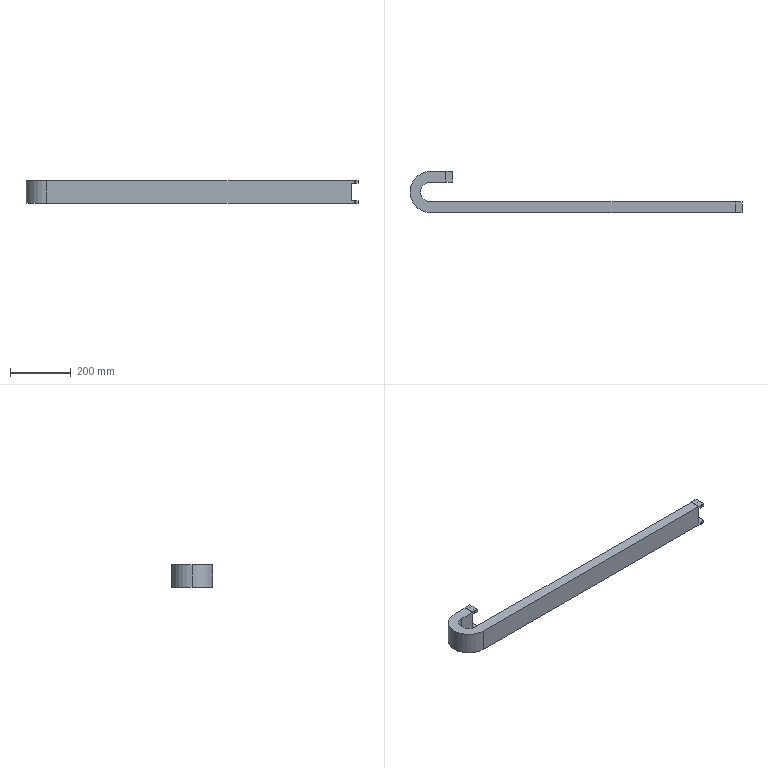Part | SolidWorks | features ICE 4, HoleWzd 2, Shell 1, Sweep 1 | 1 solid | 44 faces | box 1090 x 135 x 77 mm | volume 1433722 mm3 | plane 28 | cylinder 16 | commonest cylinder face diameters 5.5 x8 65 x2 75 x2 125 x2 135 x2
STEP:
#1=CARTESIAN_POINT('',(-938.,82.5,-36.25));
#2=VERTEX_POINT('',#1);
#3=CARTESIAN_POINT('',(-938.,82.5,-30.75));
#4=VERTEX_POINT('',#3);
#5=CARTESIAN_POINT('',(-938.,82.5,-33.5));
#6=DIRECTION('',(0.,1.,0.));
#7=DIRECTION('',(-1.,0.,0.));
#8=AXIS2_PLACEMENT_3D('',#5,#6,#7);
#9=CIRCLE('',#8,2.75);
#10=EDGE_CURVE('',#2,#4,#9,.T.);
#11=ORIENTED_EDGE('',*,*,#10,.F.);
#12=CARTESIAN_POINT('',(-938.,117.5,-36.25));
#13=VERTEX_POINT('',#12);
#14=CARTESIAN_POINT('',(-938.,117.5,-36.25));
#15=DIRECTION('',(0.,1.,0.));
#16=VECTOR('',#15,1000.);
#17=LINE('',#14,#16);
#18=EDGE_CURVE('',#2,#13,#17,.T.);
#19=ORIENTED_EDGE('',*,*,#18,.T.);
#20=CARTESIAN_POINT('',(-938.,117.5,-30.75));
#21=VERTEX_POINT('',#20);
#22=CARTESIAN_POINT('',(-938.,117.5,-33.5));
#23=DIRECTION('',(0.,1.,0.));
#24=DIRECTION('',(0.,0.,1.));
#25=AXIS2_PLACEMENT_3D('',#22,#23,#24);
#26=CIRCLE('',#25,2.75);
#27=EDGE_CURVE('',#13,#21,#26,.T.);
#28=ORIENTED_EDGE('',*,*,#27,.T.);
#29=CARTESIAN_POINT('',(-938.,117.5,-30.75));
#30=DIRECTION('',(0.,1.,0.));
#31=VECTOR('',#30,1000.);
#32=LINE('',#29,#31);
#33=EDGE_CURVE('',#4,#21,#32,.T.);
#34=ORIENTED_EDGE('',*,*,#33,.F.);
#35=EDGE_LOOP('',(#11,#19,#28,#34));
#36=FACE_OUTER_BOUND('',#35,.T.);
#37=CARTESIAN_POINT('',(-938.,117.5,-33.5));
#38=DIRECTION('',(0.,1.,0.));
#39=DIRECTION('',(0.,0.,1.));
#40=AXIS2_PLACEMENT_3D('',#37,#38,#39);
#41=CYLINDRICAL_SURFACE('',#40,2.75);
#42=ADVANCED_FACE('',(#36),#41,.F.);
#43=CARTESIAN_POINT('',(-938.,82.5,30.75));
#44=VERTEX_POINT('',#43);
#45=CARTESIAN_POINT('',(-938.,82.5,36.25));
#46=VERTEX_POINT('',#45);
#47=CARTESIAN_POINT('',(-938.,82.5,33.5));
#48=DIRECTION('',(0.,1.,0.));
#49=DIRECTION('',(-1.,0.,0.));
#50=AXIS2_PLACEMENT_3D('',#47,#48,#49);
#51=CIRCLE('',#50,2.75);
#52=EDGE_CURVE('',#44,#46,#51,.T.);
#53=ORIENTED_EDGE('',*,*,#52,.F.);
#54=CARTESIAN_POINT('',(-938.,117.5,30.75));
#55=VERTEX_POINT('',#54);
#56=CARTESIAN_POINT('',(-938.,117.5,30.75));
#57=DIRECTION('',(0.,1.,0.));
#58=VECTOR('',#57,1000.);
#59=LINE('',#56,#58);
#60=EDGE_CURVE('',#44,#55,#59,.T.);
#61=ORIENTED_EDGE('',*,*,#60,.T.);
#62=CARTESIAN_POINT('',(-938.,117.5,36.25));
#63=VERTEX_POINT('',#62);
#64=CARTESIAN_POINT('',(-938.,117.5,33.5));
#65=DIRECTION('',(0.,1.,0.));
#66=DIRECTION('',(0.,0.,1.));
#67=AXIS2_PLACEMENT_3D('',#64,#65,#66);
#68=CIRCLE('',#67,2.75);
#69=EDGE_CURVE('',#55,#63,#68,.T.);
#70=ORIENTED_EDGE('',*,*,#69,.T.);
#71=CARTESIAN_POINT('',(-938.,117.5,36.25));
#72=DIRECTION('',(0.,1.,0.));
#73=VECTOR('',#72,1000.);
#74=LINE('',#71,#73);
#75=EDGE_CURVE('',#46,#63,#74,.T.);
#76=ORIENTED_EDGE('',*,*,#75,.F.);
#77=EDGE_LOOP('',(#53,#61,#70,#76));
#78=FACE_OUTER_BOUND('',#77,.T.);
#79=CARTESIAN_POINT('',(-938.,117.5,33.5));
#80=DIRECTION('',(0.,1.,0.));
#81=DIRECTION('',(0.,0.,1.));
#82=AXIS2_PLACEMENT_3D('',#79,#80,#81);
#83=CYLINDRICAL_SURFACE('',#82,2.75);
#84=ADVANCED_FACE('',(#78),#83,.F.);
#85=CARTESIAN_POINT('',(12.,-17.5,-30.75));
#86=VERTEX_POINT('',#85);
#87=CARTESIAN_POINT('',(12.,-17.5,-36.25));
#88=VERTEX_POINT('',#87);
#89=CARTESIAN_POINT('',(12.,-17.5,-33.5));
#90=DIRECTION('',(0.,-1.,0.));
#91=DIRECTION('',(1.,0.,0.));
#92=AXIS2_PLACEMENT_3D('',#89,#90,#91);
#93=CIRCLE('',#92,2.75);
#94=EDGE_CURVE('',#86,#88,#93,.T.);
#95=ORIENTED_EDGE('',*,*,#94,.T.);
#96=CARTESIAN_POINT('',(12.,17.5,-36.25));
#97=VERTEX_POINT('',#96);
#98=CARTESIAN_POINT('',(12.,17.5,-36.25));
#99=DIRECTION('',(0.,1.,0.));
#100=VECTOR('',#99,1000.);
#101=LINE('',#98,#100);
#102=EDGE_CURVE('',#88,#97,#101,.T.);
#103=ORIENTED_EDGE('',*,*,#102,.T.);
#104=CARTESIAN_POINT('',(12.,17.5,-30.75));
#105=VERTEX_POINT('',#104);
#106=CARTESIAN_POINT('',(12.,17.5,-33.5));
#107=DIRECTION('',(0.,1.,0.));
#108=DIRECTION('',(0.,0.,1.));
#109=AXIS2_PLACEMENT_3D('',#106,#107,#108);
#110=CIRCLE('',#109,2.75);
#111=EDGE_CURVE('',#97,#105,#110,.T.);
#112=ORIENTED_EDGE('',*,*,#111,.T.);
#113=CARTESIAN_POINT('',(12.,17.5,-30.75));
#114=DIRECTION('',(0.,1.,0.));
#115=VECTOR('',#114,1000.);
#116=LINE('',#113,#115);
#117=EDGE_CURVE('',#86,#105,#116,.T.);
#118=ORIENTED_EDGE('',*,*,#117,.F.);
#119=EDGE_LOOP('',(#95,#103,#112,#118));
#120=FACE_OUTER_BOUND('',#119,.T.);
#121=CARTESIAN_POINT('',(12.,17.5,-33.5));
#122=DIRECTION('',(0.,1.,0.));
#123=DIRECTION('',(0.,0.,1.));
#124=AXIS2_PLACEMENT_3D('',#121,#122,#123);
#125=CYLINDRICAL_SURFACE('',#124,2.75);
#126=ADVANCED_FACE('',(#120),#125,.F.);
#127=CARTESIAN_POINT('',(12.,-17.5,36.25));
#128=VERTEX_POINT('',#127);
#129=CARTESIAN_POINT('',(12.,-17.5,30.75));
#130=VERTEX_POINT('',#129);
#131=CARTESIAN_POINT('',(12.,-17.5,33.5));
#132=DIRECTION('',(0.,-1.,0.));
#133=DIRECTION('',(1.,0.,0.));
#134=AXIS2_PLACEMENT_3D('',#131,#132,#133);
#135=CIRCLE('',#134,2.75);
#136=EDGE_CURVE('',#128,#130,#135,.T.);
#137=ORIENTED_EDGE('',*,*,#136,.T.);
#138=CARTESIAN_POINT('',(12.,17.5,30.75));
#139=VERTEX_POINT('',#138);
#140=CARTESIAN_POINT('',(12.,17.5,30.75));
#141=DIRECTION('',(0.,1.,0.));
#142=VECTOR('',#141,1000.);
#143=LINE('',#140,#142);
#144=EDGE_CURVE('',#130,#139,#143,.T.);
#145=ORIENTED_EDGE('',*,*,#144,.T.);
#146=CARTESIAN_POINT('',(12.,17.5,36.25));
#147=VERTEX_POINT('',#146);
#148=CARTESIAN_POINT('',(12.,17.5,33.5));
#149=DIRECTION('',(0.,1.,0.));
#150=DIRECTION('',(0.,0.,1.));
#151=AXIS2_PLACEMENT_3D('',#148,#149,#150);
#152=CIRCLE('',#151,2.75);
#153=EDGE_CURVE('',#139,#147,#152,.T.);
#154=ORIENTED_EDGE('',*,*,#153,.T.);
#155=CARTESIAN_POINT('',(12.,17.5,36.25));
#156=DIRECTION('',(0.,1.,0.));
#157=VECTOR('',#156,1000.);
#158=LINE('',#155,#157);
#159=EDGE_CURVE('',#128,#147,#158,.T.);
#160=ORIENTED_EDGE('',*,*,#159,.F.);
#161=EDGE_LOOP('',(#137,#145,#154,#160));
#162=FACE_OUTER_BOUND('',#161,.T.);
#163=CARTESIAN_POINT('',(12.,17.5,33.5));
#164=DIRECTION('',(0.,1.,0.));
#165=DIRECTION('',(0.,0.,1.));
#166=AXIS2_PLACEMENT_3D('',#163,#164,#165);
#167=CYLINDRICAL_SURFACE('',#166,2.75);
#168=ADVANCED_FACE('',(#162),#167,.F.);
#169=CARTESIAN_POINT('',(-1000.,-17.5,37.));
#170=VERTEX_POINT('',#169);
#171=CARTESIAN_POINT('',(-1067.5,50.,37.));
#172=VERTEX_POINT('',#171);
#173=CARTESIAN_POINT('',(-1000.,50.,37.));
#174=DIRECTION('',(0.,0.,-1.));
#175=DIRECTION('',(-1.,0.,0.));
#176=AXIS2_PLACEMENT_3D('',#173,#174,#175);
#177=CIRCLE('',#176,67.5);
#178=EDGE_CURVE('',#170,#172,#177,.T.);
#179=ORIENTED_EDGE('',*,*,#178,.T.);
#180=CARTESIAN_POINT('',(-1067.5,50.,-37.));
#181=VERTEX_POINT('',#180);
#182=CARTESIAN_POINT('',(-1067.5,50.,0.));
#183=DIRECTION('',(0.,0.,-1.));
#184=VECTOR('',#183,1000.);
#185=LINE('',#182,#184);
#186=EDGE_CURVE('',#172,#181,#185,.T.);
#187=ORIENTED_EDGE('',*,*,#186,.T.);
#188=CARTESIAN_POINT('',(-1000.,-17.5,-37.));
#189=VERTEX_POINT('',#188);
#190=CARTESIAN_POINT('',(-1000.,50.,-37.));
#191=DIRECTION('',(0.,0.,-1.));
#192=DIRECTION('',(-1.,0.,0.));
#193=AXIS2_PLACEMENT_3D('',#190,#191,#192);
#194=CIRCLE('',#193,67.5);
#195=EDGE_CURVE('',#189,#181,#194,.T.);
#196=ORIENTED_EDGE('',*,*,#195,.F.);
#197=CARTESIAN_POINT('',(-1000.,-17.5,-37.));
#198=DIRECTION('',(0.,0.,-1.));
#199=VECTOR('',#198,1000.);
#200=LINE('',#197,#199);
#201=EDGE_CURVE('',#170,#189,#200,.T.);
#202=ORIENTED_EDGE('',*,*,#201,.F.);
#203=EDGE_LOOP('',(#179,#187,#196,#202));
#204=FACE_OUTER_BOUND('',#203,.T.);
#205=CARTESIAN_POINT('',(-1000.,50.,0.));
#206=DIRECTION('',(0.,0.,-1.));
#207=DIRECTION('',(-1.,0.,0.));
#208=AXIS2_PLACEMENT_3D('',#205,#206,#207);
#209=CYLINDRICAL_SURFACE('',#208,67.5);
#210=ADVANCED_FACE('',(#204),#209,.T.);
#211=CARTESIAN_POINT('',(-1032.5,50.,37.));
#212=VERTEX_POINT('',#211);
#213=CARTESIAN_POINT('',(-1000.,82.5,37.));
#214=VERTEX_POINT('',#213);
#215=CARTESIAN_POINT('',(-1000.,50.,37.));
#216=DIRECTION('',(0.,0.,-1.));
#217=DIRECTION('',(-1.,0.,0.));
#218=AXIS2_PLACEMENT_3D('',#215,#216,#217);
#219=CIRCLE('',#218,32.5);
#220=EDGE_CURVE('',#212,#214,#219,.T.);
#221=ORIENTED_EDGE('',*,*,#220,.F.);
#222=CARTESIAN_POINT('',(-1032.5,50.,-37.));
#223=VERTEX_POINT('',#222);
#224=CARTESIAN_POINT('',(-1032.5,50.,0.));
#225=DIRECTION('',(0.,0.,-1.));
#226=VECTOR('',#225,1000.);
#227=LINE('',#224,#226);
#228=EDGE_CURVE('',#212,#223,#227,.T.);
#229=ORIENTED_EDGE('',*,*,#228,.T.);
#230=CARTESIAN_POINT('',(-1000.,82.5,-37.));
#231=VERTEX_POINT('',#230);
#232=CARTESIAN_POINT('',(-1000.,50.,-37.));
#233=DIRECTION('',(0.,0.,-1.));
#234=DIRECTION('',(-1.,0.,0.));
#235=AXIS2_PLACEMENT_3D('',#232,#233,#234);
#236=CIRCLE('',#235,32.5);
#237=EDGE_CURVE('',#223,#231,#236,.T.);
#238=ORIENTED_EDGE('',*,*,#237,.T.);
#239=CARTESIAN_POINT('',(-1000.,82.5,-37.));
#240=DIRECTION('',(0.,0.,1.));
#241=VECTOR('',#240,1000.);
#242=LINE('',#239,#241);
#243=EDGE_CURVE('',#231,#214,#242,.T.);
#244=ORIENTED_EDGE('',*,*,#243,.T.);
#245=EDGE_LOOP('',(#221,#229,#238,#244));
#246=FACE_OUTER_BOUND('',#245,.T.);
#247=CARTESIAN_POINT('',(-1000.,50.,0.));
#248=DIRECTION('',(0.,0.,-1.));
#249=DIRECTION('',(-1.,0.,0.));
#250=AXIS2_PLACEMENT_3D('',#247,#248,#249);
#251=CYLINDRICAL_SURFACE('',#250,32.5);
#252=ADVANCED_FACE('',(#246),#251,.F.);
#253=CARTESIAN_POINT('',(-1000.,12.5,28.5));
#254=VERTEX_POINT('',#253);
#255=CARTESIAN_POINT('',(-1037.5,50.,28.5));
#256=VERTEX_POINT('',#255);
#257=CARTESIAN_POINT('',(-1000.,50.,28.5));
#258=DIRECTION('',(0.,0.,-1.));
#259=DIRECTION('',(-1.,0.,0.));
#260=AXIS2_PLACEMENT_3D('',#257,#258,#259);
#261=CIRCLE('',#260,37.5);
#262=EDGE_CURVE('',#254,#256,#261,.T.);
#263=ORIENTED_EDGE('',*,*,#262,.T.);
#264=CARTESIAN_POINT('',(-1037.5,50.,-28.5));
#265=VERTEX_POINT('',#264);
#266=CARTESIAN_POINT('',(-1037.5,50.,0.));
#267=DIRECTION('',(0.,0.,-1.));
#268=VECTOR('',#267,1000.);
#269=LINE('',#266,#268);
#270=EDGE_CURVE('',#256,#265,#269,.T.);
#271=ORIENTED_EDGE('',*,*,#270,.T.);
#272=CARTESIAN_POINT('',(-1000.,12.5,-28.5));
#273=VERTEX_POINT('',#272);
#274=CARTESIAN_POINT('',(-1000.,50.,-28.5));
#275=DIRECTION('',(0.,0.,-1.));
#276=DIRECTION('',(-1.,0.,0.));
#277=AXIS2_PLACEMENT_3D('',#274,#275,#276);
#278=CIRCLE('',#277,37.5);
#279=EDGE_CURVE('',#273,#265,#278,.T.);
#280=ORIENTED_EDGE('',*,*,#279,.F.);
#281=CARTESIAN_POINT('',(-1000.,12.5,-28.5));
#282=DIRECTION('',(0.,0.,1.));
#283=VECTOR('',#282,1000.);
#284=LINE('',#281,#283);
#285=EDGE_CURVE('',#273,#254,#284,.T.);
#286=ORIENTED_EDGE('',*,*,#285,.T.);
#287=EDGE_LOOP('',(#263,#271,#280,#286));
#288=FACE_OUTER_BOUND('',#287,.T.);
#289=CARTESIAN_POINT('',(-1000.,50.,0.));
#290=DIRECTION('',(0.,0.,-1.));
#291=DIRECTION('',(-1.,0.,0.));
#292=AXIS2_PLACEMENT_3D('',#289,#290,#291);
#293=CYLINDRICAL_SURFACE('',#292,37.5);
#294=ADVANCED_FACE('',(#288),#293,.T.);
#295=CARTESIAN_POINT('',(-1062.5,50.,28.5));
#296=VERTEX_POINT('',#295);
#297=CARTESIAN_POINT('',(-1000.,112.5,28.5));
#298=VERTEX_POINT('',#297);
#299=CARTESIAN_POINT('',(-1000.,50.,28.5));
#300=DIRECTION('',(0.,0.,-1.));
#301=DIRECTION('',(-1.,0.,0.));
#302=AXIS2_PLACEMENT_3D('',#299,#300,#301);
#303=CIRCLE('',#302,62.5);
#304=EDGE_CURVE('',#296,#298,#303,.T.);
#305=ORIENTED_EDGE('',*,*,#304,.F.);
#306=CARTESIAN_POINT('',(-1062.5,50.,-28.5));
#307=VERTEX_POINT('',#306);
#308=CARTESIAN_POINT('',(-1062.5,50.,0.));
#309=DIRECTION('',(0.,0.,-1.));
#310=VECTOR('',#309,1000.);
#311=LINE('',#308,#310);
#312=EDGE_CURVE('',#296,#307,#311,.T.);
#313=ORIENTED_EDGE('',*,*,#312,.T.);
#314=CARTESIAN_POINT('',(-1000.,112.5,-28.5));
#315=VERTEX_POINT('',#314);
#316=CARTESIAN_POINT('',(-1000.,50.,-28.5));
#317=DIRECTION('',(0.,0.,-1.));
#318=DIRECTION('',(-1.,0.,0.));
#319=AXIS2_PLACEMENT_3D('',#316,#317,#318);
#320=CIRCLE('',#319,62.5);
#321=EDGE_CURVE('',#307,#315,#320,.T.);
#322=ORIENTED_EDGE('',*,*,#321,.T.);
#323=CARTESIAN_POINT('',(-1000.,112.5,-28.5));
#324=DIRECTION('',(0.,0.,-1.));
#325=VECTOR('',#324,1000.);
#326=LINE('',#323,#325);
#327=EDGE_CURVE('',#298,#315,#326,.T.);
#328=ORIENTED_EDGE('',*,*,#327,.F.);
#329=EDGE_LOOP('',(#305,#313,#322,#328));
#330=FACE_OUTER_BOUND('',#329,.T.);
#331=CARTESIAN_POINT('',(-1000.,50.,0.));
#332=DIRECTION('',(0.,0.,-1.));
#333=DIRECTION('',(-1.,0.,0.));
#334=AXIS2_PLACEMENT_3D('',#331,#332,#333);
#335=CYLINDRICAL_SURFACE('',#334,62.5);
#336=ADVANCED_FACE('',(#330),#335,.F.);
#337=CARTESIAN_POINT('',(-928.,117.5,28.5));
#338=VERTEX_POINT('',#337);
#339=CARTESIAN_POINT('',(-928.,82.5,28.5));
#340=VERTEX_POINT('',#339);
#341=CARTESIAN_POINT('',(-928.,87.5,28.5));
#342=DIRECTION('',(0.,-1.,0.));
#343=VECTOR('',#342,1000.);
#344=LINE('',#341,#343);
#345=EDGE_CURVE('',#338,#340,#344,.T.);
#346=ORIENTED_EDGE('',*,*,#345,.F.);
#347=CARTESIAN_POINT('',(-928.,117.5,38.5));
#348=VERTEX_POINT('',#347);
#349=CARTESIAN_POINT('',(-928.,117.5,38.5));
#350=DIRECTION('',(0.,0.,1.));
#351=VECTOR('',#350,1000.);
#352=LINE('',#349,#351);
#353=EDGE_CURVE('',#338,#348,#352,.T.);
#354=ORIENTED_EDGE('',*,*,#353,.T.);
#355=CARTESIAN_POINT('',(-928.,82.5,38.5));
#356=VERTEX_POINT('',#355);
#357=CARTESIAN_POINT('',(-928.,117.5,38.5));
#358=DIRECTION('',(0.,-1.,0.));
#359=VECTOR('',#358,1000.);
#360=LINE('',#357,#359);
#361=EDGE_CURVE('',#348,#356,#360,.T.);
#362=ORIENTED_EDGE('',*,*,#361,.T.);
#363=CARTESIAN_POINT('',(-928.,82.5,38.5));
#364=DIRECTION('',(0.,0.,-1.));
#365=VECTOR('',#364,1000.);
#366=LINE('',#363,#365);
#367=EDGE_CURVE('',#356,#340,#366,.T.);
#368=ORIENTED_EDGE('',*,*,#367,.T.);
#369=EDGE_LOOP('',(#346,#354,#362,#368));
#370=FACE_OUTER_BOUND('',#369,.T.);
#371=CARTESIAN_POINT('',(-928.,0.,0.));
#372=DIRECTION('',(1.,0.,0.));
#373=DIRECTION('',(0.,0.,-1.));
#374=AXIS2_PLACEMENT_3D('',#371,#372,#373);
#375=PLANE('',#374);
#376=ADVANCED_FACE('',(#370),#375,.T.);
#377=CARTESIAN_POINT('',(22.,17.5,28.5));
#378=VERTEX_POINT('',#377);
#379=CARTESIAN_POINT('',(22.,-17.5,28.5));
#380=VERTEX_POINT('',#379);
#381=CARTESIAN_POINT('',(22.,12.5,28.5));
#382=DIRECTION('',(0.,-1.,0.));
#383=VECTOR('',#382,1000.);
#384=LINE('',#381,#383);
#385=EDGE_CURVE('',#378,#380,#384,.T.);
#386=ORIENTED_EDGE('',*,*,#385,.F.);
#387=CARTESIAN_POINT('',(22.,17.5,38.5));
#388=VERTEX_POINT('',#387);
#389=CARTESIAN_POINT('',(22.,17.5,38.5));
#390=DIRECTION('',(0.,0.,1.));
#391=VECTOR('',#390,1000.);
#392=LINE('',#389,#391);
#393=EDGE_CURVE('',#378,#388,#392,.T.);
#394=ORIENTED_EDGE('',*,*,#393,.T.);
#395=CARTESIAN_POINT('',(22.,-17.5,38.5));
#396=VERTEX_POINT('',#395);
#397=CARTESIAN_POINT('',(22.,17.5,38.5));
#398=DIRECTION('',(0.,-1.,0.));
#399=VECTOR('',#398,1000.);
#400=LINE('',#397,#399);
#401=EDGE_CURVE('',#388,#396,#400,.T.);
#402=ORIENTED_EDGE('',*,*,#401,.T.);
#403=CARTESIAN_POINT('',(22.,-17.5,38.5));
#404=DIRECTION('',(0.,0.,-1.));
#405=VECTOR('',#404,1000.);
#406=LINE('',#403,#405);
#407=EDGE_CURVE('',#396,#380,#406,.T.);
#408=ORIENTED_EDGE('',*,*,#407,.T.);
#409=EDGE_LOOP('',(#386,#394,#402,#408));
#410=FACE_OUTER_BOUND('',#409,.T.);
#411=CARTESIAN_POINT('',(22.,0.,0.));
#412=DIRECTION('',(1.,0.,0.));
#413=DIRECTION('',(0.,0.,-1.));
#414=AXIS2_PLACEMENT_3D('',#411,#412,#413);
#415=PLANE('',#414);
#416=ADVANCED_FACE('',(#410),#415,.T.);
#417=CARTESIAN_POINT('',(-950.,112.5,28.5));
#418=VERTEX_POINT('',#417);
#419=CARTESIAN_POINT('',(-950.,112.5,-28.5));
#420=VERTEX_POINT('',#419);
#421=CARTESIAN_POINT('',(-950.,112.5,-28.5));
#422=DIRECTION('',(0.,0.,-1.));
#423=VECTOR('',#422,1000.);
#424=LINE('',#421,#423);
#425=EDGE_CURVE('',#418,#420,#424,.T.);
#426=ORIENTED_EDGE('',*,*,#425,.F.);
#427=CARTESIAN_POINT('',(-1000.,112.5,28.5));
#428=DIRECTION('',(1.,0.,0.));
#429=VECTOR('',#428,1000.);
#430=LINE('',#427,#429);
#431=EDGE_CURVE('',#298,#418,#430,.T.);
#432=ORIENTED_EDGE('',*,*,#431,.F.);
#433=ORIENTED_EDGE('',*,*,#327,.T.);
#434=CARTESIAN_POINT('',(-1000.,112.5,-28.5));
#435=DIRECTION('',(1.,0.,0.));
#436=VECTOR('',#435,1000.);
#437=LINE('',#434,#436);
#438=EDGE_CURVE('',#315,#420,#437,.T.);
#439=ORIENTED_EDGE('',*,*,#438,.T.);
#440=EDGE_LOOP('',(#426,#432,#433,#439));
#441=FACE_OUTER_BOUND('',#440,.T.);
#442=CARTESIAN_POINT('',(-1000.,112.5,-28.5));
#443=DIRECTION('',(0.,-1.,0.));
#444=DIRECTION('',(1.,0.,0.));
#445=AXIS2_PLACEMENT_3D('',#442,#443,#444);
#446=PLANE('',#445);
#447=ADVANCED_FACE('',(#441),#446,.T.);
#448=CARTESIAN_POINT('',(-950.,87.5,-28.5));
#449=VERTEX_POINT('',#448);
#450=CARTESIAN_POINT('',(-950.,87.5,28.5));
#451=VERTEX_POINT('',#450);
#452=CARTESIAN_POINT('',(-950.,87.5,-28.5));
#453=DIRECTION('',(0.,0.,1.));
#454=VECTOR('',#453,1000.);
#455=LINE('',#452,#454);
#456=EDGE_CURVE('',#449,#451,#455,.T.);
#457=ORIENTED_EDGE('',*,*,#456,.F.);
#458=CARTESIAN_POINT('',(-1000.,87.5,-28.5));
#459=VERTEX_POINT('',#458);
#460=CARTESIAN_POINT('',(-1000.,87.5,-28.5));
#461=DIRECTION('',(1.,0.,0.));
#462=VECTOR('',#461,1000.);
#463=LINE('',#460,#462);
#464=EDGE_CURVE('',#459,#449,#463,.T.);
#465=ORIENTED_EDGE('',*,*,#464,.F.);
#466=CARTESIAN_POINT('',(-1000.,87.5,28.5));
#467=VERTEX_POINT('',#466);
#468=CARTESIAN_POINT('',(-1000.,87.5,-28.5));
#469=DIRECTION('',(0.,0.,1.));
#470=VECTOR('',#469,1000.);
#471=LINE('',#468,#470);
#472=EDGE_CURVE('',#459,#467,#471,.T.);
#473=ORIENTED_EDGE('',*,*,#472,.T.);
#474=CARTESIAN_POINT('',(-1000.,87.5,28.5));
#475=DIRECTION('',(1.,0.,0.));
#476=VECTOR('',#475,1000.);
#477=LINE('',#474,#476);
#478=EDGE_CURVE('',#467,#451,#477,.T.);
#479=ORIENTED_EDGE('',*,*,#478,.T.);
#480=EDGE_LOOP('',(#457,#465,#473,#479));
#481=FACE_OUTER_BOUND('',#480,.T.);
#482=CARTESIAN_POINT('',(-1000.,87.5,-28.5));
#483=DIRECTION('',(0.,1.,0.));
#484=DIRECTION('',(-1.,0.,0.));
#485=AXIS2_PLACEMENT_3D('',#482,#483,#484);
#486=PLANE('',#485);
#487=ADVANCED_FACE('',(#481),#486,.T.);
#488=CARTESIAN_POINT('',(-938.,82.5,-33.5));
#489=DIRECTION('',(0.,1.,0.));
#490=DIRECTION('',(-1.,0.,0.));
#491=AXIS2_PLACEMENT_3D('',#488,#489,#490);
#492=CIRCLE('',#491,2.75);
#493=EDGE_CURVE('',#4,#2,#492,.T.);
#494=ORIENTED_EDGE('',*,*,#493,.T.);
#495=ORIENTED_EDGE('',*,*,#10,.T.);
#496=EDGE_LOOP('',(#494,#495));
#497=FACE_BOUND('',#496,.T.);
#498=CARTESIAN_POINT('',(-938.,82.5,33.5));
#499=DIRECTION('',(0.,1.,0.));
#500=DIRECTION('',(-1.,0.,0.));
#501=AXIS2_PLACEMENT_3D('',#498,#499,#500);
#502=CIRCLE('',#501,2.75);
#503=EDGE_CURVE('',#46,#44,#502,.T.);
#504=ORIENTED_EDGE('',*,*,#503,.T.);
#505=ORIENTED_EDGE('',*,*,#52,.T.);
#506=EDGE_LOOP('',(#504,#505));
#507=FACE_BOUND('',#506,.T.);
#508=CARTESIAN_POINT('',(-950.,82.5,-28.5));
#509=VERTEX_POINT('',#508);
#510=CARTESIAN_POINT('',(-950.,82.5,28.5));
#511=VERTEX_POINT('',#510);
#512=CARTESIAN_POINT('',(-950.,82.5,-37.));
#513=DIRECTION('',(0.,0.,1.));
#514=VECTOR('',#513,1000.);
#515=LINE('',#512,#514);
#516=EDGE_CURVE('',#509,#511,#515,.T.);
#517=ORIENTED_EDGE('',*,*,#516,.T.);
#518=CARTESIAN_POINT('',(-1000.,82.5,28.5));
#519=DIRECTION('',(1.,0.,0.));
#520=VECTOR('',#519,1000.);
#521=LINE('',#518,#520);
#522=EDGE_CURVE('',#511,#340,#521,.T.);
#523=ORIENTED_EDGE('',*,*,#522,.T.);
#524=ORIENTED_EDGE('',*,*,#367,.F.);
#525=CARTESIAN_POINT('',(-950.,82.5,38.5));
#526=VERTEX_POINT('',#525);
#527=CARTESIAN_POINT('',(-928.,82.5,38.5));
#528=DIRECTION('',(-1.,0.,0.));
#529=VECTOR('',#528,1000.);
#530=LINE('',#527,#529);
#531=EDGE_CURVE('',#356,#526,#530,.T.);
#532=ORIENTED_EDGE('',*,*,#531,.T.);
#533=CARTESIAN_POINT('',(-950.,82.5,37.));
#534=VERTEX_POINT('',#533);
#535=CARTESIAN_POINT('',(-950.,82.5,38.5));
#536=DIRECTION('',(0.,0.,-1.));
#537=VECTOR('',#536,1000.);
#538=LINE('',#535,#537);
#539=EDGE_CURVE('',#526,#534,#538,.T.);
#540=ORIENTED_EDGE('',*,*,#539,.T.);
#541=CARTESIAN_POINT('',(-1000.,82.5,37.));
#542=DIRECTION('',(1.,0.,0.));
#543=VECTOR('',#542,1000.);
#544=LINE('',#541,#543);
#545=EDGE_CURVE('',#214,#534,#544,.T.);
#546=ORIENTED_EDGE('',*,*,#545,.F.);
#547=ORIENTED_EDGE('',*,*,#243,.F.);
#548=CARTESIAN_POINT('',(-950.,82.5,-37.));
#549=VERTEX_POINT('',#548);
#550=CARTESIAN_POINT('',(-1000.,82.5,-37.));
#551=DIRECTION('',(1.,0.,0.));
#552=VECTOR('',#551,1000.);
#553=LINE('',#550,#552);
#554=EDGE_CURVE('',#231,#549,#553,.T.);
#555=ORIENTED_EDGE('',*,*,#554,.T.);
#556=CARTESIAN_POINT('',(-950.,82.5,-38.5));
#557=VERTEX_POINT('',#556);
#558=CARTESIAN_POINT('',(-950.,82.5,38.5));
#559=DIRECTION('',(0.,0.,-1.));
#560=VECTOR('',#559,1000.);
#561=LINE('',#558,#560);
#562=EDGE_CURVE('',#549,#557,#561,.T.);
#563=ORIENTED_EDGE('',*,*,#562,.T.);
#564=CARTESIAN_POINT('',(-928.,82.5,-38.5));
#565=VERTEX_POINT('',#564);
#566=CARTESIAN_POINT('',(-928.,82.5,-38.5));
#567=DIRECTION('',(-1.,0.,0.));
#568=VECTOR('',#567,1000.);
#569=LINE('',#566,#568);
#570=EDGE_CURVE('',#565,#557,#569,.T.);
#571=ORIENTED_EDGE('',*,*,#570,.F.);
#572=CARTESIAN_POINT('',(-928.,82.5,-28.5));
#573=VERTEX_POINT('',#572);
#574=CARTESIAN_POINT('',(-928.,82.5,38.5));
#575=DIRECTION('',(0.,0.,-1.));
#576=VECTOR('',#575,1000.);
#577=LINE('',#574,#576);
#578=EDGE_CURVE('',#573,#565,#577,.T.);
#579=ORIENTED_EDGE('',*,*,#578,.F.);
#580=CARTESIAN_POINT('',(-1000.,82.5,-28.5));
#581=DIRECTION('',(-1.,0.,0.));
#582=VECTOR('',#581,1000.);
#583=LINE('',#580,#582);
#584=EDGE_CURVE('',#573,#509,#583,.T.);
#585=ORIENTED_EDGE('',*,*,#584,.T.);
#586=EDGE_LOOP('',(#517,#523,#524,#532,#540,#546,#547,#555,#563,#571,#579,#585));
#587=FACE_OUTER_BOUND('',#586,.T.);
#588=CARTESIAN_POINT('',(-1000.,82.5,-37.));
#589=DIRECTION('',(0.,1.,0.));
#590=DIRECTION('',(-1.,0.,0.));
#591=AXIS2_PLACEMENT_3D('',#588,#589,#590);
#592=PLANE('',#591);
#593=ADVANCED_FACE('',(#497,#507,#587),#592,.F.);
#594=CARTESIAN_POINT('',(-938.,117.5,-33.5));
#595=DIRECTION('',(0.,1.,0.));
#596=DIRECTION('',(0.,0.,1.));
#597=AXIS2_PLACEMENT_3D('',#594,#595,#596);
#598=CIRCLE('',#597,2.75);
#599=EDGE_CURVE('',#21,#13,#598,.T.);
#600=ORIENTED_EDGE('',*,*,#599,.F.);
#601=ORIENTED_EDGE('',*,*,#27,.F.);
#602=EDGE_LOOP('',(#600,#601));
#603=FACE_BOUND('',#602,.T.);
#604=CARTESIAN_POINT('',(-938.,117.5,33.5));
#605=DIRECTION('',(0.,1.,0.));
#606=DIRECTION('',(0.,0.,1.));
#607=AXIS2_PLACEMENT_3D('',#604,#605,#606);
#608=CIRCLE('',#607,2.75);
#609=EDGE_CURVE('',#63,#55,#608,.T.);
#610=ORIENTED_EDGE('',*,*,#609,.F.);
#611=ORIENTED_EDGE('',*,*,#69,.F.);
#612=EDGE_LOOP('',(#610,#611));
#613=FACE_BOUND('',#612,.T.);
#614=ORIENTED_EDGE('',*,*,#353,.F.);
#615=CARTESIAN_POINT('',(-950.,117.5,28.5));
#616=VERTEX_POINT('',#615);
#617=CARTESIAN_POINT('',(-950.,117.5,28.5));
#618=DIRECTION('',(1.,0.,0.));
#619=VECTOR('',#618,1000.);
#620=LINE('',#617,#619);
#621=EDGE_CURVE('',#616,#338,#620,.T.);
#622=ORIENTED_EDGE('',*,*,#621,.F.);
#623=CARTESIAN_POINT('',(-950.,117.5,-28.5));
#624=VERTEX_POINT('',#623);
#625=CARTESIAN_POINT('',(-950.,117.5,-28.5));
#626=DIRECTION('',(0.,0.,1.));
#627=VECTOR('',#626,1000.);
#628=LINE('',#625,#627);
#629=EDGE_CURVE('',#624,#616,#628,.T.);
#630=ORIENTED_EDGE('',*,*,#629,.F.);
#631=CARTESIAN_POINT('',(-928.,117.5,-28.5));
#632=VERTEX_POINT('',#631);
#633=CARTESIAN_POINT('',(-950.,117.5,-28.5));
#634=DIRECTION('',(-1.,0.,0.));
#635=VECTOR('',#634,1000.);
#636=LINE('',#633,#635);
#637=EDGE_CURVE('',#632,#624,#636,.T.);
#638=ORIENTED_EDGE('',*,*,#637,.F.);
#639=CARTESIAN_POINT('',(-928.,117.5,-38.5));
#640=VERTEX_POINT('',#639);
#641=CARTESIAN_POINT('',(-928.,117.5,38.5));
#642=DIRECTION('',(0.,0.,1.));
#643=VECTOR('',#642,1000.);
#644=LINE('',#641,#643);
#645=EDGE_CURVE('',#640,#632,#644,.T.);
#646=ORIENTED_EDGE('',*,*,#645,.F.);
#647=CARTESIAN_POINT('',(-950.,117.5,-38.5));
#648=VERTEX_POINT('',#647);
#649=CARTESIAN_POINT('',(-928.,117.5,-38.5));
#650=DIRECTION('',(-1.,0.,0.));
#651=VECTOR('',#650,1000.);
#652=LINE('',#649,#651);
#653=EDGE_CURVE('',#640,#648,#652,.T.);
#654=ORIENTED_EDGE('',*,*,#653,.T.);
#655=CARTESIAN_POINT('',(-950.,117.5,-37.));
#656=VERTEX_POINT('',#655);
#657=CARTESIAN_POINT('',(-950.,117.5,38.5));
#658=DIRECTION('',(0.,0.,1.));
#659=VECTOR('',#658,1000.);
#660=LINE('',#657,#659);
#661=EDGE_CURVE('',#648,#656,#660,.T.);
#662=ORIENTED_EDGE('',*,*,#661,.T.);
#663=CARTESIAN_POINT('',(-1000.,117.5,-37.));
#664=VERTEX_POINT('',#663);
#665=CARTESIAN_POINT('',(-1000.,117.5,-37.));
#666=DIRECTION('',(1.,0.,0.));
#667=VECTOR('',#666,1000.);
#668=LINE('',#665,#667);
#669=EDGE_CURVE('',#664,#656,#668,.T.);
#670=ORIENTED_EDGE('',*,*,#669,.F.);
#671=CARTESIAN_POINT('',(-1000.,117.5,37.));
#672=VERTEX_POINT('',#671);
#673=CARTESIAN_POINT('',(-1000.,117.5,-37.));
#674=DIRECTION('',(0.,0.,-1.));
#675=VECTOR('',#674,1000.);
#676=LINE('',#673,#675);
#677=EDGE_CURVE('',#672,#664,#676,.T.);
#678=ORIENTED_EDGE('',*,*,#677,.F.);
#679=CARTESIAN_POINT('',(-950.,117.5,37.));
#680=VERTEX_POINT('',#679);
#681=CARTESIAN_POINT('',(-1000.,117.5,37.));
#682=DIRECTION('',(1.,0.,0.));
#683=VECTOR('',#682,1000.);
#684=LINE('',#681,#683);
#685=EDGE_CURVE('',#672,#680,#684,.T.);
#686=ORIENTED_EDGE('',*,*,#685,.T.);
#687=CARTESIAN_POINT('',(-950.,117.5,38.5));
#688=VERTEX_POINT('',#687);
#689=CARTESIAN_POINT('',(-950.,117.5,38.5));
#690=DIRECTION('',(0.,0.,1.));
#691=VECTOR('',#690,1000.);
#692=LINE('',#689,#691);
#693=EDGE_CURVE('',#680,#688,#692,.T.);
#694=ORIENTED_EDGE('',*,*,#693,.T.);
#695=CARTESIAN_POINT('',(-928.,117.5,38.5));
#696=DIRECTION('',(-1.,0.,0.));
#697=VECTOR('',#696,1000.);
#698=LINE('',#695,#697);
#699=EDGE_CURVE('',#348,#688,#698,.T.);
#700=ORIENTED_EDGE('',*,*,#699,.F.);
#701=EDGE_LOOP('',(#614,#622,#630,#638,#646,#654,#662,#670,#678,#686,#694,#700));
#702=FACE_OUTER_BOUND('',#701,.T.);
#703=CARTESIAN_POINT('',(-1000.,117.5,-37.));
#704=DIRECTION('',(0.,-1.,0.));
#705=DIRECTION('',(1.,0.,0.));
#706=AXIS2_PLACEMENT_3D('',#703,#704,#705);
#707=PLANE('',#706);
#708=ADVANCED_FACE('',(#603,#613,#702),#707,.F.);
#709=ORIENTED_EDGE('',*,*,#312,.F.);
#710=CARTESIAN_POINT('',(-1000.,-12.5,28.5));
#711=VERTEX_POINT('',#710);
#712=CARTESIAN_POINT('',(-1000.,50.,28.5));
#713=DIRECTION('',(0.,0.,-1.));
#714=DIRECTION('',(-1.,0.,0.));
#715=AXIS2_PLACEMENT_3D('',#712,#713,#714);
#716=CIRCLE('',#715,62.5);
#717=EDGE_CURVE('',#711,#296,#716,.T.);
#718=ORIENTED_EDGE('',*,*,#717,.F.);
#719=CARTESIAN_POINT('',(-1000.,-12.5,-28.5));
#720=VERTEX_POINT('',#719);
#721=CARTESIAN_POINT('',(-1000.,-12.5,-28.5));
#722=DIRECTION('',(0.,0.,-1.));
#723=VECTOR('',#722,1000.);
#724=LINE('',#721,#723);
#725=EDGE_CURVE('',#711,#720,#724,.T.);
#726=ORIENTED_EDGE('',*,*,#725,.T.);
#727=CARTESIAN_POINT('',(-1000.,50.,-28.5));
#728=DIRECTION('',(0.,0.,-1.));
#729=DIRECTION('',(-1.,0.,0.));
#730=AXIS2_PLACEMENT_3D('',#727,#728,#729);
#731=CIRCLE('',#730,62.5);
#732=EDGE_CURVE('',#720,#307,#731,.T.);
#733=ORIENTED_EDGE('',*,*,#732,.T.);
#734=EDGE_LOOP('',(#709,#718,#726,#733));
#735=FACE_OUTER_BOUND('',#734,.T.);
#736=CARTESIAN_POINT('',(-1000.,50.,0.));
#737=DIRECTION('',(0.,0.,-1.));
#738=DIRECTION('',(-1.,0.,0.));
#739=AXIS2_PLACEMENT_3D('',#736,#737,#738);
#740=CYLINDRICAL_SURFACE('',#739,62.5);
#741=ADVANCED_FACE('',(#735),#740,.F.);
#742=ORIENTED_EDGE('',*,*,#270,.F.);
#743=CARTESIAN_POINT('',(-1000.,50.,28.5));
#744=DIRECTION('',(0.,0.,-1.));
#745=DIRECTION('',(-1.,0.,0.));
#746=AXIS2_PLACEMENT_3D('',#743,#744,#745);
#747=CIRCLE('',#746,37.5);
#748=EDGE_CURVE('',#256,#467,#747,.T.);
#749=ORIENTED_EDGE('',*,*,#748,.T.);
#750=ORIENTED_EDGE('',*,*,#472,.F.);
#751=CARTESIAN_POINT('',(-1000.,50.,-28.5));
#752=DIRECTION('',(0.,0.,-1.));
#753=DIRECTION('',(-1.,0.,0.));
#754=AXIS2_PLACEMENT_3D('',#751,#752,#753);
#755=CIRCLE('',#754,37.5);
#756=EDGE_CURVE('',#265,#459,#755,.T.);
#757=ORIENTED_EDGE('',*,*,#756,.F.);
#758=EDGE_LOOP('',(#742,#749,#750,#757));
#759=FACE_OUTER_BOUND('',#758,.T.);
#760=CARTESIAN_POINT('',(-1000.,50.,0.));
#761=DIRECTION('',(0.,0.,-1.));
#762=DIRECTION('',(-1.,0.,0.));
#763=AXIS2_PLACEMENT_3D('',#760,#761,#762);
#764=CYLINDRICAL_SURFACE('',#763,37.5);
#765=ADVANCED_FACE('',(#759),#764,.T.);
#766=ORIENTED_EDGE('',*,*,#228,.F.);
#767=CARTESIAN_POINT('',(-1000.,17.5,37.));
#768=VERTEX_POINT('',#767);
#769=CARTESIAN_POINT('',(-1000.,50.,37.));
#770=DIRECTION('',(0.,0.,-1.));
#771=DIRECTION('',(-1.,0.,0.));
#772=AXIS2_PLACEMENT_3D('',#769,#770,#771);
#773=CIRCLE('',#772,32.5);
#774=EDGE_CURVE('',#768,#212,#773,.T.);
#775=ORIENTED_EDGE('',*,*,#774,.F.);
#776=CARTESIAN_POINT('',(-1000.,17.5,-37.));
#777=VERTEX_POINT('',#776);
#778=CARTESIAN_POINT('',(-1000.,17.5,-37.));
#779=DIRECTION('',(0.,0.,1.));
#780=VECTOR('',#779,1000.);
#781=LINE('',#778,#780);
#782=EDGE_CURVE('',#777,#768,#781,.T.);
#783=ORIENTED_EDGE('',*,*,#782,.F.);
#784=CARTESIAN_POINT('',(-1000.,50.,-37.));
#785=DIRECTION('',(0.,0.,-1.));
#786=DIRECTION('',(-1.,0.,0.));
#787=AXIS2_PLACEMENT_3D('',#784,#785,#786);
#788=CIRCLE('',#787,32.5);
#789=EDGE_CURVE('',#777,#223,#788,.T.);
#790=ORIENTED_EDGE('',*,*,#789,.T.);
#791=EDGE_LOOP('',(#766,#775,#783,#790));
#792=FACE_OUTER_BOUND('',#791,.T.);
#793=CARTESIAN_POINT('',(-1000.,50.,0.));
#794=DIRECTION('',(0.,0.,-1.));
#795=DIRECTION('',(-1.,0.,0.));
#796=AXIS2_PLACEMENT_3D('',#793,#794,#795);
#797=CYLINDRICAL_SURFACE('',#796,32.5);
#798=ADVANCED_FACE('',(#792),#797,.F.);
#799=ORIENTED_EDGE('',*,*,#186,.F.);
#800=CARTESIAN_POINT('',(-1000.,50.,37.));
#801=DIRECTION('',(0.,0.,-1.));
#802=DIRECTION('',(-1.,0.,0.));
#803=AXIS2_PLACEMENT_3D('',#800,#801,#802);
#804=CIRCLE('',#803,67.5);
#805=EDGE_CURVE('',#172,#672,#804,.T.);
#806=ORIENTED_EDGE('',*,*,#805,.T.);
#807=ORIENTED_EDGE('',*,*,#677,.T.);
#808=CARTESIAN_POINT('',(-1000.,50.,-37.));
#809=DIRECTION('',(0.,0.,-1.));
#810=DIRECTION('',(-1.,0.,0.));
#811=AXIS2_PLACEMENT_3D('',#808,#809,#810);
#812=CIRCLE('',#811,67.5);
#813=EDGE_CURVE('',#181,#664,#812,.T.);
#814=ORIENTED_EDGE('',*,*,#813,.F.);
#815=EDGE_LOOP('',(#799,#806,#807,#814));
#816=FACE_OUTER_BOUND('',#815,.T.);
#817=CARTESIAN_POINT('',(-1000.,50.,0.));
#818=DIRECTION('',(0.,0.,-1.));
#819=DIRECTION('',(-1.,0.,0.));
#820=AXIS2_PLACEMENT_3D('',#817,#818,#819);
#821=CYLINDRICAL_SURFACE('',#820,67.5);
#822=ADVANCED_FACE('',(#816),#821,.T.);
#823=ORIENTED_EDGE('',*,*,#431,.T.);
#824=CARTESIAN_POINT('',(-950.,68.5,28.5));
#825=DIRECTION('',(0.,1.,0.));
#826=VECTOR('',#825,1000.);
#827=LINE('',#824,#826);
#828=EDGE_CURVE('',#418,#616,#827,.T.);
#829=ORIENTED_EDGE('',*,*,#828,.T.);
#830=ORIENTED_EDGE('',*,*,#621,.T.);
#831=ORIENTED_EDGE('',*,*,#345,.T.);
#832=ORIENTED_EDGE('',*,*,#522,.F.);
#833=CARTESIAN_POINT('',(-950.,68.5,28.5));
#834=DIRECTION('',(0.,1.,0.));
#835=VECTOR('',#834,1000.);
#836=LINE('',#833,#835);
#837=EDGE_CURVE('',#511,#451,#836,.T.);
#838=ORIENTED_EDGE('',*,*,#837,.T.);
#839=ORIENTED_EDGE('',*,*,#478,.F.);
#840=ORIENTED_EDGE('',*,*,#748,.F.);
#841=ORIENTED_EDGE('',*,*,#262,.F.);
#842=CARTESIAN_POINT('',(0.,12.5,28.5));
#843=VERTEX_POINT('',#842);
#844=CARTESIAN_POINT('',(-1000.,12.5,28.5));
#845=DIRECTION('',(1.,0.,0.));
#846=VECTOR('',#845,1000.);
#847=LINE('',#844,#846);
#848=EDGE_CURVE('',#254,#843,#847,.T.);
#849=ORIENTED_EDGE('',*,*,#848,.T.);
#850=CARTESIAN_POINT('',(0.,17.5,28.5));
#851=VERTEX_POINT('',#850);
#852=CARTESIAN_POINT('',(0.,-17.5,28.5));
#853=DIRECTION('',(0.,1.,0.));
#854=VECTOR('',#853,1000.);
#855=LINE('',#852,#854);
#856=EDGE_CURVE('',#843,#851,#855,.T.);
#857=ORIENTED_EDGE('',*,*,#856,.T.);
#858=CARTESIAN_POINT('',(0.,17.5,28.5));
#859=DIRECTION('',(1.,0.,0.));
#860=VECTOR('',#859,1000.);
#861=LINE('',#858,#860);
#862=EDGE_CURVE('',#851,#378,#861,.T.);
#863=ORIENTED_EDGE('',*,*,#862,.T.);
#864=ORIENTED_EDGE('',*,*,#385,.T.);
#865=CARTESIAN_POINT('',(0.,-17.5,28.5));
#866=VERTEX_POINT('',#865);
#867=CARTESIAN_POINT('',(-1000.,-17.5,28.5));
#868=DIRECTION('',(-1.,0.,0.));
#869=VECTOR('',#868,1000.);
#870=LINE('',#867,#869);
#871=EDGE_CURVE('',#380,#866,#870,.T.);
#872=ORIENTED_EDGE('',*,*,#871,.T.);
#873=CARTESIAN_POINT('',(0.,-12.5,28.5));
#874=VERTEX_POINT('',#873);
#875=CARTESIAN_POINT('',(0.,-17.5,28.5));
#876=DIRECTION('',(0.,1.,0.));
#877=VECTOR('',#876,1000.);
#878=LINE('',#875,#877);
#879=EDGE_CURVE('',#866,#874,#878,.T.);
#880=ORIENTED_EDGE('',*,*,#879,.T.);
#881=CARTESIAN_POINT('',(-1000.,-12.5,28.5));
#882=DIRECTION('',(1.,0.,0.));
#883=VECTOR('',#882,1000.);
#884=LINE('',#881,#883);
#885=EDGE_CURVE('',#711,#874,#884,.T.);
#886=ORIENTED_EDGE('',*,*,#885,.F.);
#887=ORIENTED_EDGE('',*,*,#717,.T.);
#888=ORIENTED_EDGE('',*,*,#304,.T.);
#889=EDGE_LOOP('',(#823,#829,#830,#831,#832,#838,#839,#840,#841,#849,#857,#863,#864,#872,#880,#886,#887,#888));
#890=FACE_OUTER_BOUND('',#889,.T.);
#891=CARTESIAN_POINT('',(-1000.,12.5,28.5));
#892=DIRECTION('',(0.,0.,1.));
#893=DIRECTION('',(0.,-1.,0.));
#894=AXIS2_PLACEMENT_3D('',#891,#892,#893);
#895=PLANE('',#894);
#896=ADVANCED_FACE('',(#890),#895,.F.);
#897=ORIENTED_EDGE('',*,*,#885,.T.);
#898=CARTESIAN_POINT('',(0.,-12.5,-28.5));
#899=VERTEX_POINT('',#898);
#900=CARTESIAN_POINT('',(0.,-12.5,-28.5));
#901=DIRECTION('',(0.,0.,-1.));
#902=VECTOR('',#901,1000.);
#903=LINE('',#900,#902);
#904=EDGE_CURVE('',#874,#899,#903,.T.);
#905=ORIENTED_EDGE('',*,*,#904,.T.);
#906=CARTESIAN_POINT('',(-1000.,-12.5,-28.5));
#907=DIRECTION('',(1.,0.,0.));
#908=VECTOR('',#907,1000.);
#909=LINE('',#906,#908);
#910=EDGE_CURVE('',#720,#899,#909,.T.);
#911=ORIENTED_EDGE('',*,*,#910,.F.);
#912=ORIENTED_EDGE('',*,*,#725,.F.);
#913=EDGE_LOOP('',(#897,#905,#911,#912));
#914=FACE_OUTER_BOUND('',#913,.T.);
#915=CARTESIAN_POINT('',(-1000.,-12.5,-28.5));
#916=DIRECTION('',(0.,-1.,0.));
#917=DIRECTION('',(1.,0.,0.));
#918=AXIS2_PLACEMENT_3D('',#915,#916,#917);
#919=PLANE('',#918);
#920=ADVANCED_FACE('',(#914),#919,.F.);
#921=ORIENTED_EDGE('',*,*,#464,.T.);
#922=CARTESIAN_POINT('',(-950.,68.5,-28.5));
#923=DIRECTION('',(0.,1.,0.));
#924=VECTOR('',#923,1000.);
#925=LINE('',#922,#924);
#926=EDGE_CURVE('',#509,#449,#925,.T.);
#927=ORIENTED_EDGE('',*,*,#926,.F.);
#928=ORIENTED_EDGE('',*,*,#584,.F.);
#929=CARTESIAN_POINT('',(-928.,112.5,-28.5));
#930=DIRECTION('',(0.,1.,0.));
#931=VECTOR('',#930,1000.);
#932=LINE('',#929,#931);
#933=EDGE_CURVE('',#573,#632,#932,.T.);
#934=ORIENTED_EDGE('',*,*,#933,.T.);
#935=ORIENTED_EDGE('',*,*,#637,.T.);
#936=CARTESIAN_POINT('',(-950.,68.5,-28.5));
#937=DIRECTION('',(0.,1.,0.));
#938=VECTOR('',#937,1000.);
#939=LINE('',#936,#938);
#940=EDGE_CURVE('',#420,#624,#939,.T.);
#941=ORIENTED_EDGE('',*,*,#940,.F.);
#942=ORIENTED_EDGE('',*,*,#438,.F.);
#943=ORIENTED_EDGE('',*,*,#321,.F.);
#944=ORIENTED_EDGE('',*,*,#732,.F.);
#945=ORIENTED_EDGE('',*,*,#910,.T.);
#946=CARTESIAN_POINT('',(0.,-17.5,-28.5));
#947=VERTEX_POINT('',#946);
#948=CARTESIAN_POINT('',(0.,-17.5,-28.5));
#949=DIRECTION('',(0.,1.,0.));
#950=VECTOR('',#949,1000.);
#951=LINE('',#948,#950);
#952=EDGE_CURVE('',#947,#899,#951,.T.);
#953=ORIENTED_EDGE('',*,*,#952,.F.);
#954=CARTESIAN_POINT('',(22.,-17.5,-28.5));
#955=VERTEX_POINT('',#954);
#956=CARTESIAN_POINT('',(-1000.,-17.5,-28.5));
#957=DIRECTION('',(1.,0.,0.));
#958=VECTOR('',#957,1000.);
#959=LINE('',#956,#958);
#960=EDGE_CURVE('',#947,#955,#959,.T.);
#961=ORIENTED_EDGE('',*,*,#960,.T.);
#962=CARTESIAN_POINT('',(22.,17.5,-28.5));
#963=VERTEX_POINT('',#962);
#964=CARTESIAN_POINT('',(22.,-12.5,-28.5));
#965=DIRECTION('',(0.,1.,0.));
#966=VECTOR('',#965,1000.);
#967=LINE('',#964,#966);
#968=EDGE_CURVE('',#955,#963,#967,.T.);
#969=ORIENTED_EDGE('',*,*,#968,.T.);
#970=CARTESIAN_POINT('',(0.,17.5,-28.5));
#971=VERTEX_POINT('',#970);
#972=CARTESIAN_POINT('',(0.,17.5,-28.5));
#973=DIRECTION('',(-1.,0.,0.));
#974=VECTOR('',#973,1000.);
#975=LINE('',#972,#974);
#976=EDGE_CURVE('',#963,#971,#975,.T.);
#977=ORIENTED_EDGE('',*,*,#976,.T.);
#978=CARTESIAN_POINT('',(0.,12.5,-28.5));
#979=VERTEX_POINT('',#978);
#980=CARTESIAN_POINT('',(0.,-17.5,-28.5));
#981=DIRECTION('',(0.,1.,0.));
#982=VECTOR('',#981,1000.);
#983=LINE('',#980,#982);
#984=EDGE_CURVE('',#979,#971,#983,.T.);
#985=ORIENTED_EDGE('',*,*,#984,.F.);
#986=CARTESIAN_POINT('',(-1000.,12.5,-28.5));
#987=DIRECTION('',(1.,0.,0.));
#988=VECTOR('',#987,1000.);
#989=LINE('',#986,#988);
#990=EDGE_CURVE('',#273,#979,#989,.T.);
#991=ORIENTED_EDGE('',*,*,#990,.F.);
#992=ORIENTED_EDGE('',*,*,#279,.T.);
#993=ORIENTED_EDGE('',*,*,#756,.T.);
#994=EDGE_LOOP('',(#921,#927,#928,#934,#935,#941,#942,#943,#944,#945,#953,#961,#969,#977,#985,#991,#992,#993));
#995=FACE_OUTER_BOUND('',#994,.T.);
#996=CARTESIAN_POINT('',(-1000.,12.5,-28.5));
#997=DIRECTION('',(0.,0.,-1.));
#998=DIRECTION('',(-1.,0.,0.));
#999=AXIS2_PLACEMENT_3D('',#996,#997,#998);
#1000=PLANE('',#999);
#1001=ADVANCED_FACE('',(#995),#1000,.F.);
#1002=CARTESIAN_POINT('',(0.,17.5,37.));
#1003=VERTEX_POINT('',#1002);
#1004=CARTESIAN_POINT('',(0.,-17.5,37.));
#1005=VERTEX_POINT('',#1004);
#1006=CARTESIAN_POINT('',(0.,17.5,37.));
#1007=DIRECTION('',(0.,-1.,0.));
#1008=VECTOR('',#1007,1000.);
#1009=LINE('',#1006,#1008);
#1010=EDGE_CURVE('',#1003,#1005,#1009,.T.);
#1011=ORIENTED_EDGE('',*,*,#1010,.F.);
#1012=CARTESIAN_POINT('',(-1000.,17.5,37.));
#1013=DIRECTION('',(1.,0.,0.));
#1014=VECTOR('',#1013,1000.);
#1015=LINE('',#1012,#1014);
#1016=EDGE_CURVE('',#768,#1003,#1015,.T.);
#1017=ORIENTED_EDGE('',*,*,#1016,.F.);
#1018=ORIENTED_EDGE('',*,*,#774,.T.);
#1019=ORIENTED_EDGE('',*,*,#220,.T.);
#1020=ORIENTED_EDGE('',*,*,#545,.T.);
#1021=CARTESIAN_POINT('',(-950.,82.5,37.));
#1022=DIRECTION('',(0.,1.,0.));
#1023=VECTOR('',#1022,1000.);
#1024=LINE('',#1021,#1023);
#1025=EDGE_CURVE('',#534,#680,#1024,.T.);
#1026=ORIENTED_EDGE('',*,*,#1025,.T.);
#1027=ORIENTED_EDGE('',*,*,#685,.F.);
#1028=ORIENTED_EDGE('',*,*,#805,.F.);
#1029=ORIENTED_EDGE('',*,*,#178,.F.);
#1030=CARTESIAN_POINT('',(-1000.,-17.5,37.));
#1031=DIRECTION('',(1.,0.,0.));
#1032=VECTOR('',#1031,1000.);
#1033=LINE('',#1030,#1032);
#1034=EDGE_CURVE('',#170,#1005,#1033,.T.);
#1035=ORIENTED_EDGE('',*,*,#1034,.T.);
#1036=EDGE_LOOP('',(#1011,#1017,#1018,#1019,#1020,#1026,#1027,#1028,#1029,#1035));
#1037=FACE_OUTER_BOUND('',#1036,.T.);
#1038=CARTESIAN_POINT('',(-1000.,17.5,37.));
#1039=DIRECTION('',(0.,0.,1.));
#1040=DIRECTION('',(0.,-1.,0.));
#1041=AXIS2_PLACEMENT_3D('',#1038,#1039,#1040);
#1042=PLANE('',#1041);
#1043=ADVANCED_FACE('',(#1037),#1042,.T.);
#1044=CARTESIAN_POINT('',(12.,17.5,-33.5));
#1045=DIRECTION('',(0.,1.,0.));
#1046=DIRECTION('',(0.,0.,1.));
#1047=AXIS2_PLACEMENT_3D('',#1044,#1045,#1046);
#1048=CIRCLE('',#1047,2.75);
#1049=EDGE_CURVE('',#105,#97,#1048,.T.);
#1050=ORIENTED_EDGE('',*,*,#1049,.F.);
#1051=ORIENTED_EDGE('',*,*,#111,.F.);
#1052=EDGE_LOOP('',(#1050,#1051));
#1053=FACE_BOUND('',#1052,.T.);
#1054=CARTESIAN_POINT('',(12.,17.5,33.5));
#1055=DIRECTION('',(0.,1.,0.));
#1056=DIRECTION('',(0.,0.,1.));
#1057=AXIS2_PLACEMENT_3D('',#1054,#1055,#1056);
#1058=CIRCLE('',#1057,2.75);
#1059=EDGE_CURVE('',#147,#139,#1058,.T.);
#1060=ORIENTED_EDGE('',*,*,#1059,.F.);
#1061=ORIENTED_EDGE('',*,*,#153,.F.);
#1062=EDGE_LOOP('',(#1060,#1061));
#1063=FACE_BOUND('',#1062,.T.);
#1064=ORIENTED_EDGE('',*,*,#862,.F.);
#1065=CARTESIAN_POINT('',(0.,17.5,-28.5));
#1066=DIRECTION('',(0.,0.,1.));
#1067=VECTOR('',#1066,1000.);
#1068=LINE('',#1065,#1067);
#1069=EDGE_CURVE('',#971,#851,#1068,.T.);
#1070=ORIENTED_EDGE('',*,*,#1069,.F.);
#1071=ORIENTED_EDGE('',*,*,#976,.F.);
#1072=CARTESIAN_POINT('',(22.,17.5,-38.5));
#1073=VERTEX_POINT('',#1072);
#1074=CARTESIAN_POINT('',(22.,17.5,38.5));
#1075=DIRECTION('',(0.,0.,1.));
#1076=VECTOR('',#1075,1000.);
#1077=LINE('',#1074,#1076);
#1078=EDGE_CURVE('',#1073,#963,#1077,.T.);
#1079=ORIENTED_EDGE('',*,*,#1078,.F.);
#1080=CARTESIAN_POINT('',(0.,17.5,-38.5));
#1081=VERTEX_POINT('',#1080);
#1082=CARTESIAN_POINT('',(22.,17.5,-38.5));
#1083=DIRECTION('',(-1.,0.,0.));
#1084=VECTOR('',#1083,1000.);
#1085=LINE('',#1082,#1084);
#1086=EDGE_CURVE('',#1073,#1081,#1085,.T.);
#1087=ORIENTED_EDGE('',*,*,#1086,.T.);
#1088=CARTESIAN_POINT('',(0.,17.5,-37.));
#1089=VERTEX_POINT('',#1088);
#1090=CARTESIAN_POINT('',(0.,17.5,38.5));
#1091=DIRECTION('',(0.,0.,1.));
#1092=VECTOR('',#1091,1000.);
#1093=LINE('',#1090,#1092);
#1094=EDGE_CURVE('',#1081,#1089,#1093,.T.);
#1095=ORIENTED_EDGE('',*,*,#1094,.T.);
#1096=CARTESIAN_POINT('',(-1000.,17.5,-37.));
#1097=DIRECTION('',(1.,0.,0.));
#1098=VECTOR('',#1097,1000.);
#1099=LINE('',#1096,#1098);
#1100=EDGE_CURVE('',#777,#1089,#1099,.T.);
#1101=ORIENTED_EDGE('',*,*,#1100,.F.);
#1102=ORIENTED_EDGE('',*,*,#782,.T.);
#1103=ORIENTED_EDGE('',*,*,#1016,.T.);
#1104=CARTESIAN_POINT('',(0.,17.5,38.5));
#1105=VERTEX_POINT('',#1104);
#1106=CARTESIAN_POINT('',(0.,17.5,38.5));
#1107=DIRECTION('',(0.,0.,1.));
#1108=VECTOR('',#1107,1000.);
#1109=LINE('',#1106,#1108);
#1110=EDGE_CURVE('',#1003,#1105,#1109,.T.);
#1111=ORIENTED_EDGE('',*,*,#1110,.T.);
#1112=CARTESIAN_POINT('',(22.,17.5,38.5));
#1113=DIRECTION('',(-1.,0.,0.));
#1114=VECTOR('',#1113,1000.);
#1115=LINE('',#1112,#1114);
#1116=EDGE_CURVE('',#388,#1105,#1115,.T.);
#1117=ORIENTED_EDGE('',*,*,#1116,.F.);
#1118=ORIENTED_EDGE('',*,*,#393,.F.);
#1119=EDGE_LOOP('',(#1064,#1070,#1071,#1079,#1087,#1095,#1101,#1102,#1103,#1111,#1117,#1118));
#1120=FACE_OUTER_BOUND('',#1119,.T.);
#1121=CARTESIAN_POINT('',(-1000.,17.5,-37.));
#1122=DIRECTION('',(0.,1.,0.));
#1123=DIRECTION('',(0.,0.,1.));
#1124=AXIS2_PLACEMENT_3D('',#1121,#1122,#1123);
#1125=PLANE('',#1124);
#1126=ADVANCED_FACE('',(#1053,#1063,#1120),#1125,.T.);
#1127=CARTESIAN_POINT('',(0.,-17.5,-37.));
#1128=VERTEX_POINT('',#1127);
#1129=CARTESIAN_POINT('',(0.,17.5,-37.));
#1130=DIRECTION('',(0.,1.,0.));
#1131=VECTOR('',#1130,1000.);
#1132=LINE('',#1129,#1131);
#1133=EDGE_CURVE('',#1128,#1089,#1132,.T.);
#1134=ORIENTED_EDGE('',*,*,#1133,.F.);
#1135=CARTESIAN_POINT('',(-1000.,-17.5,-37.));
#1136=DIRECTION('',(1.,0.,0.));
#1137=VECTOR('',#1136,1000.);
#1138=LINE('',#1135,#1137);
#1139=EDGE_CURVE('',#189,#1128,#1138,.T.);
#1140=ORIENTED_EDGE('',*,*,#1139,.F.);
#1141=ORIENTED_EDGE('',*,*,#195,.T.);
#1142=ORIENTED_EDGE('',*,*,#813,.T.);
#1143=ORIENTED_EDGE('',*,*,#669,.T.);
#1144=CARTESIAN_POINT('',(-950.,82.5,-37.));
#1145=DIRECTION('',(0.,-1.,0.));
#1146=VECTOR('',#1145,1000.);
#1147=LINE('',#1144,#1146);
#1148=EDGE_CURVE('',#656,#549,#1147,.T.);
#1149=ORIENTED_EDGE('',*,*,#1148,.T.);
#1150=ORIENTED_EDGE('',*,*,#554,.F.);
#1151=ORIENTED_EDGE('',*,*,#237,.F.);
#1152=ORIENTED_EDGE('',*,*,#789,.F.);
#1153=ORIENTED_EDGE('',*,*,#1100,.T.);
#1154=EDGE_LOOP('',(#1134,#1140,#1141,#1142,#1143,#1149,#1150,#1151,#1152,#1153));
#1155=FACE_OUTER_BOUND('',#1154,.T.);
#1156=CARTESIAN_POINT('',(-1000.,17.5,-37.));
#1157=DIRECTION('',(0.,0.,-1.));
#1158=DIRECTION('',(-1.,0.,0.));
#1159=AXIS2_PLACEMENT_3D('',#1156,#1157,#1158);
#1160=PLANE('',#1159);
#1161=ADVANCED_FACE('',(#1155),#1160,.T.);
#1162=ORIENTED_EDGE('',*,*,#94,.F.);
#1163=CARTESIAN_POINT('',(12.,-17.5,-33.5));
#1164=DIRECTION('',(0.,-1.,0.));
#1165=DIRECTION('',(1.,0.,0.));
#1166=AXIS2_PLACEMENT_3D('',#1163,#1164,#1165);
#1167=CIRCLE('',#1166,2.75);
#1168=EDGE_CURVE('',#88,#86,#1167,.T.);
#1169=ORIENTED_EDGE('',*,*,#1168,.F.);
#1170=EDGE_LOOP('',(#1162,#1169));
#1171=FACE_BOUND('',#1170,.T.);
#1172=ORIENTED_EDGE('',*,*,#136,.F.);
#1173=CARTESIAN_POINT('',(12.,-17.5,33.5));
#1174=DIRECTION('',(0.,-1.,0.));
#1175=DIRECTION('',(1.,0.,0.));
#1176=AXIS2_PLACEMENT_3D('',#1173,#1174,#1175);
#1177=CIRCLE('',#1176,2.75);
#1178=EDGE_CURVE('',#130,#128,#1177,.T.);
#1179=ORIENTED_EDGE('',*,*,#1178,.F.);
#1180=EDGE_LOOP('',(#1172,#1179));
#1181=FACE_BOUND('',#1180,.T.);
#1182=ORIENTED_EDGE('',*,*,#871,.F.);
#1183=ORIENTED_EDGE('',*,*,#407,.F.);
#1184=CARTESIAN_POINT('',(0.,-17.5,38.5));
#1185=VERTEX_POINT('',#1184);
#1186=CARTESIAN_POINT('',(22.,-17.5,38.5));
#1187=DIRECTION('',(-1.,0.,0.));
#1188=VECTOR('',#1187,1000.);
#1189=LINE('',#1186,#1188);
#1190=EDGE_CURVE('',#396,#1185,#1189,.T.);
#1191=ORIENTED_EDGE('',*,*,#1190,.T.);
#1192=CARTESIAN_POINT('',(0.,-17.5,38.5));
#1193=DIRECTION('',(0.,0.,-1.));
#1194=VECTOR('',#1193,1000.);
#1195=LINE('',#1192,#1194);
#1196=EDGE_CURVE('',#1185,#1005,#1195,.T.);
#1197=ORIENTED_EDGE('',*,*,#1196,.T.);
#1198=ORIENTED_EDGE('',*,*,#1034,.F.);
#1199=ORIENTED_EDGE('',*,*,#201,.T.);
#1200=ORIENTED_EDGE('',*,*,#1139,.T.);
#1201=CARTESIAN_POINT('',(0.,-17.5,-38.5));
#1202=VERTEX_POINT('',#1201);
#1203=CARTESIAN_POINT('',(0.,-17.5,38.5));
#1204=DIRECTION('',(0.,0.,-1.));
#1205=VECTOR('',#1204,1000.);
#1206=LINE('',#1203,#1205);
#1207=EDGE_CURVE('',#1128,#1202,#1206,.T.);
#1208=ORIENTED_EDGE('',*,*,#1207,.T.);
#1209=CARTESIAN_POINT('',(22.,-17.5,-38.5));
#1210=VERTEX_POINT('',#1209);
#1211=CARTESIAN_POINT('',(22.,-17.5,-38.5));
#1212=DIRECTION('',(-1.,0.,0.));
#1213=VECTOR('',#1212,1000.);
#1214=LINE('',#1211,#1213);
#1215=EDGE_CURVE('',#1210,#1202,#1214,.T.);
#1216=ORIENTED_EDGE('',*,*,#1215,.F.);
#1217=CARTESIAN_POINT('',(22.,-17.5,38.5));
#1218=DIRECTION('',(0.,0.,-1.));
#1219=VECTOR('',#1218,1000.);
#1220=LINE('',#1217,#1219);
#1221=EDGE_CURVE('',#955,#1210,#1220,.T.);
#1222=ORIENTED_EDGE('',*,*,#1221,.F.);
#1223=ORIENTED_EDGE('',*,*,#960,.F.);
#1224=CARTESIAN_POINT('',(0.,-17.5,-37.));
#1225=DIRECTION('',(0.,0.,-1.));
#1226=VECTOR('',#1225,1000.);
#1227=LINE('',#1224,#1226);
#1228=EDGE_CURVE('',#866,#947,#1227,.T.);
#1229=ORIENTED_EDGE('',*,*,#1228,.F.);
#1230=EDGE_LOOP('',(#1182,#1183,#1191,#1197,#1198,#1199,#1200,#1208,#1216,#1222,#1223,#1229));
#1231=FACE_OUTER_BOUND('',#1230,.T.);
#1232=CARTESIAN_POINT('',(-1000.,-17.5,-37.));
#1233=DIRECTION('',(0.,-1.,0.));
#1234=DIRECTION('',(1.,0.,0.));
#1235=AXIS2_PLACEMENT_3D('',#1232,#1233,#1234);
#1236=PLANE('',#1235);
#1237=ADVANCED_FACE('',(#1171,#1181,#1231),#1236,.T.);
#1238=ORIENTED_EDGE('',*,*,#990,.T.);
#1239=CARTESIAN_POINT('',(0.,12.5,-28.5));
#1240=DIRECTION('',(0.,0.,1.));
#1241=VECTOR('',#1240,1000.);
#1242=LINE('',#1239,#1241);
#1243=EDGE_CURVE('',#979,#843,#1242,.T.);
#1244=ORIENTED_EDGE('',*,*,#1243,.T.);
#1245=ORIENTED_EDGE('',*,*,#848,.F.);
#1246=ORIENTED_EDGE('',*,*,#285,.F.);
#1247=EDGE_LOOP('',(#1238,#1244,#1245,#1246));
#1248=FACE_OUTER_BOUND('',#1247,.T.);
#1249=CARTESIAN_POINT('',(-1000.,12.5,-28.5));
#1250=DIRECTION('',(0.,1.,0.));
#1251=DIRECTION('',(-1.,0.,0.));
#1252=AXIS2_PLACEMENT_3D('',#1249,#1250,#1251);
#1253=PLANE('',#1252);
#1254=ADVANCED_FACE('',(#1248),#1253,.F.);
#1255=ORIENTED_EDGE('',*,*,#1110,.F.);
#1256=ORIENTED_EDGE('',*,*,#1010,.T.);
#1257=ORIENTED_EDGE('',*,*,#1196,.F.);
#1258=CARTESIAN_POINT('',(0.,17.5,38.5));
#1259=DIRECTION('',(0.,-1.,0.));
#1260=VECTOR('',#1259,1000.);
#1261=LINE('',#1258,#1260);
#1262=EDGE_CURVE('',#1105,#1185,#1261,.T.);
#1263=ORIENTED_EDGE('',*,*,#1262,.F.);
#1264=EDGE_LOOP('',(#1255,#1256,#1257,#1263));
#1265=FACE_OUTER_BOUND('',#1264,.T.);
#1266=CARTESIAN_POINT('',(0.,0.,0.));
#1267=DIRECTION('',(1.,0.,0.));
#1268=DIRECTION('',(0.,0.,-1.));
#1269=AXIS2_PLACEMENT_3D('',#1266,#1267,#1268);
#1270=PLANE('',#1269);
#1271=ADVANCED_FACE('',(#1265),#1270,.F.);
#1272=ORIENTED_EDGE('',*,*,#1207,.F.);
#1273=ORIENTED_EDGE('',*,*,#1133,.T.);
#1274=ORIENTED_EDGE('',*,*,#1094,.F.);
#1275=CARTESIAN_POINT('',(0.,17.5,-38.5));
#1276=DIRECTION('',(0.,1.,0.));
#1277=VECTOR('',#1276,1000.);
#1278=LINE('',#1275,#1277);
#1279=EDGE_CURVE('',#1202,#1081,#1278,.T.);
#1280=ORIENTED_EDGE('',*,*,#1279,.F.);
#1281=EDGE_LOOP('',(#1272,#1273,#1274,#1280));
#1282=FACE_OUTER_BOUND('',#1281,.T.);
#1283=CARTESIAN_POINT('',(0.,0.,0.));
#1284=DIRECTION('',(1.,0.,0.));
#1285=DIRECTION('',(0.,0.,-1.));
#1286=AXIS2_PLACEMENT_3D('',#1283,#1284,#1285);
#1287=PLANE('',#1286);
#1288=ADVANCED_FACE('',(#1282),#1287,.F.);
#1289=ORIENTED_EDGE('',*,*,#968,.F.);
#1290=ORIENTED_EDGE('',*,*,#1221,.T.);
#1291=CARTESIAN_POINT('',(22.,17.5,-38.5));
#1292=DIRECTION('',(0.,1.,0.));
#1293=VECTOR('',#1292,1000.);
#1294=LINE('',#1291,#1293);
#1295=EDGE_CURVE('',#1210,#1073,#1294,.T.);
#1296=ORIENTED_EDGE('',*,*,#1295,.T.);
#1297=ORIENTED_EDGE('',*,*,#1078,.T.);
#1298=EDGE_LOOP('',(#1289,#1290,#1296,#1297));
#1299=FACE_OUTER_BOUND('',#1298,.T.);
#1300=CARTESIAN_POINT('',(22.,0.,0.));
#1301=DIRECTION('',(1.,0.,0.));
#1302=DIRECTION('',(0.,0.,-1.));
#1303=AXIS2_PLACEMENT_3D('',#1300,#1301,#1302);
#1304=PLANE('',#1303);
#1305=ADVANCED_FACE('',(#1299),#1304,.T.);
#1306=ORIENTED_EDGE('',*,*,#1279,.T.);
#1307=ORIENTED_EDGE('',*,*,#1086,.F.);
#1308=ORIENTED_EDGE('',*,*,#1295,.F.);
#1309=ORIENTED_EDGE('',*,*,#1215,.T.);
#1310=EDGE_LOOP('',(#1306,#1307,#1308,#1309));
#1311=FACE_OUTER_BOUND('',#1310,.T.);
#1312=CARTESIAN_POINT('',(22.,17.5,-38.5));
#1313=DIRECTION('',(0.,0.,1.));
#1314=DIRECTION('',(1.,0.,0.));
#1315=AXIS2_PLACEMENT_3D('',#1312,#1313,#1314);
#1316=PLANE('',#1315);
#1317=ADVANCED_FACE('',(#1311),#1316,.F.);
#1318=ORIENTED_EDGE('',*,*,#1262,.T.);
#1319=ORIENTED_EDGE('',*,*,#1190,.F.);
#1320=ORIENTED_EDGE('',*,*,#401,.F.);
#1321=ORIENTED_EDGE('',*,*,#1116,.T.);
#1322=EDGE_LOOP('',(#1318,#1319,#1320,#1321));
#1323=FACE_OUTER_BOUND('',#1322,.T.);
#1324=CARTESIAN_POINT('',(22.,17.5,38.5));
#1325=DIRECTION('',(0.,0.,-1.));
#1326=DIRECTION('',(-1.,0.,0.));
#1327=AXIS2_PLACEMENT_3D('',#1324,#1325,#1326);
#1328=PLANE('',#1327);
#1329=ADVANCED_FACE('',(#1323),#1328,.F.);
#1330=ORIENTED_EDGE('',*,*,#984,.T.);
#1331=ORIENTED_EDGE('',*,*,#1069,.T.);
#1332=ORIENTED_EDGE('',*,*,#856,.F.);
#1333=ORIENTED_EDGE('',*,*,#1243,.F.);
#1334=EDGE_LOOP('',(#1330,#1331,#1332,#1333));
#1335=FACE_OUTER_BOUND('',#1334,.T.);
#1336=CARTESIAN_POINT('',(0.,-17.5,-28.5));
#1337=DIRECTION('',(-1.,0.,0.));
#1338=DIRECTION('',(0.,-1.,0.));
#1339=AXIS2_PLACEMENT_3D('',#1336,#1337,#1338);
#1340=PLANE('',#1339);
#1341=ADVANCED_FACE('',(#1335),#1340,.F.);
#1342=ORIENTED_EDGE('',*,*,#879,.F.);
#1343=ORIENTED_EDGE('',*,*,#1228,.T.);
#1344=ORIENTED_EDGE('',*,*,#952,.T.);
#1345=ORIENTED_EDGE('',*,*,#904,.F.);
#1346=EDGE_LOOP('',(#1342,#1343,#1344,#1345));
#1347=FACE_OUTER_BOUND('',#1346,.T.);
#1348=CARTESIAN_POINT('',(0.,-17.5,-28.5));
#1349=DIRECTION('',(-1.,0.,0.));
#1350=DIRECTION('',(0.,-1.,0.));
#1351=AXIS2_PLACEMENT_3D('',#1348,#1349,#1350);
#1352=PLANE('',#1351);
#1353=ADVANCED_FACE('',(#1347),#1352,.F.);
#1354=ORIENTED_EDGE('',*,*,#144,.F.);
#1355=ORIENTED_EDGE('',*,*,#1178,.T.);
#1356=ORIENTED_EDGE('',*,*,#159,.T.);
#1357=ORIENTED_EDGE('',*,*,#1059,.T.);
#1358=EDGE_LOOP('',(#1354,#1355,#1356,#1357));
#1359=FACE_OUTER_BOUND('',#1358,.T.);
#1360=CARTESIAN_POINT('',(12.,17.5,33.5));
#1361=DIRECTION('',(0.,1.,0.));
#1362=DIRECTION('',(0.,0.,1.));
#1363=AXIS2_PLACEMENT_3D('',#1360,#1361,#1362);
#1364=CYLINDRICAL_SURFACE('',#1363,2.75);
#1365=ADVANCED_FACE('',(#1359),#1364,.F.);
#1366=ORIENTED_EDGE('',*,*,#102,.F.);
#1367=ORIENTED_EDGE('',*,*,#1168,.T.);
#1368=ORIENTED_EDGE('',*,*,#117,.T.);
#1369=ORIENTED_EDGE('',*,*,#1049,.T.);
#1370=EDGE_LOOP('',(#1366,#1367,#1368,#1369));
#1371=FACE_OUTER_BOUND('',#1370,.T.);
#1372=CARTESIAN_POINT('',(12.,17.5,-33.5));
#1373=DIRECTION('',(0.,1.,0.));
#1374=DIRECTION('',(0.,0.,1.));
#1375=AXIS2_PLACEMENT_3D('',#1372,#1373,#1374);
#1376=CYLINDRICAL_SURFACE('',#1375,2.75);
#1377=ADVANCED_FACE('',(#1371),#1376,.F.);
#1378=ORIENTED_EDGE('',*,*,#1025,.F.);
#1379=ORIENTED_EDGE('',*,*,#539,.F.);
#1380=CARTESIAN_POINT('',(-950.,117.5,38.5));
#1381=DIRECTION('',(0.,-1.,0.));
#1382=VECTOR('',#1381,1000.);
#1383=LINE('',#1380,#1382);
#1384=EDGE_CURVE('',#688,#526,#1383,.T.);
#1385=ORIENTED_EDGE('',*,*,#1384,.F.);
#1386=ORIENTED_EDGE('',*,*,#693,.F.);
#1387=EDGE_LOOP('',(#1378,#1379,#1385,#1386));
#1388=FACE_OUTER_BOUND('',#1387,.T.);
#1389=CARTESIAN_POINT('',(-950.,0.,0.));
#1390=DIRECTION('',(1.,0.,0.));
#1391=DIRECTION('',(0.,0.,-1.));
#1392=AXIS2_PLACEMENT_3D('',#1389,#1390,#1391);
#1393=PLANE('',#1392);
#1394=ADVANCED_FACE('',(#1388),#1393,.F.);
#1395=ORIENTED_EDGE('',*,*,#933,.F.);
#1396=ORIENTED_EDGE('',*,*,#578,.T.);
#1397=CARTESIAN_POINT('',(-928.,117.5,-38.5));
#1398=DIRECTION('',(0.,1.,0.));
#1399=VECTOR('',#1398,1000.);
#1400=LINE('',#1397,#1399);
#1401=EDGE_CURVE('',#565,#640,#1400,.T.);
#1402=ORIENTED_EDGE('',*,*,#1401,.T.);
#1403=ORIENTED_EDGE('',*,*,#645,.T.);
#1404=EDGE_LOOP('',(#1395,#1396,#1402,#1403));
#1405=FACE_OUTER_BOUND('',#1404,.T.);
#1406=CARTESIAN_POINT('',(-928.,0.,0.));
#1407=DIRECTION('',(1.,0.,0.));
#1408=DIRECTION('',(0.,0.,-1.));
#1409=AXIS2_PLACEMENT_3D('',#1406,#1407,#1408);
#1410=PLANE('',#1409);
#1411=ADVANCED_FACE('',(#1405),#1410,.T.);
#1412=ORIENTED_EDGE('',*,*,#1148,.F.);
#1413=ORIENTED_EDGE('',*,*,#661,.F.);
#1414=CARTESIAN_POINT('',(-950.,117.5,-38.5));
#1415=DIRECTION('',(0.,1.,0.));
#1416=VECTOR('',#1415,1000.);
#1417=LINE('',#1414,#1416);
#1418=EDGE_CURVE('',#557,#648,#1417,.T.);
#1419=ORIENTED_EDGE('',*,*,#1418,.F.);
#1420=ORIENTED_EDGE('',*,*,#562,.F.);
#1421=EDGE_LOOP('',(#1412,#1413,#1419,#1420));
#1422=FACE_OUTER_BOUND('',#1421,.T.);
#1423=CARTESIAN_POINT('',(-950.,0.,0.));
#1424=DIRECTION('',(1.,0.,0.));
#1425=DIRECTION('',(0.,0.,-1.));
#1426=AXIS2_PLACEMENT_3D('',#1423,#1424,#1425);
#1427=PLANE('',#1426);
#1428=ADVANCED_FACE('',(#1422),#1427,.F.);
#1429=ORIENTED_EDGE('',*,*,#1418,.T.);
#1430=ORIENTED_EDGE('',*,*,#653,.F.);
#1431=ORIENTED_EDGE('',*,*,#1401,.F.);
#1432=ORIENTED_EDGE('',*,*,#570,.T.);
#1433=EDGE_LOOP('',(#1429,#1430,#1431,#1432));
#1434=FACE_OUTER_BOUND('',#1433,.T.);
#1435=CARTESIAN_POINT('',(-928.,117.5,-38.5));
#1436=DIRECTION('',(0.,0.,1.));
#1437=DIRECTION('',(0.,-1.,0.));
#1438=AXIS2_PLACEMENT_3D('',#1435,#1436,#1437);
#1439=PLANE('',#1438);
#1440=ADVANCED_FACE('',(#1434),#1439,.F.);
#1441=ORIENTED_EDGE('',*,*,#1384,.T.);
#1442=ORIENTED_EDGE('',*,*,#531,.F.);
#1443=ORIENTED_EDGE('',*,*,#361,.F.);
#1444=ORIENTED_EDGE('',*,*,#699,.T.);
#1445=EDGE_LOOP('',(#1441,#1442,#1443,#1444));
#1446=FACE_OUTER_BOUND('',#1445,.T.);
#1447=CARTESIAN_POINT('',(-928.,117.5,38.5));
#1448=DIRECTION('',(0.,0.,-1.));
#1449=DIRECTION('',(-1.,0.,0.));
#1450=AXIS2_PLACEMENT_3D('',#1447,#1448,#1449);
#1451=PLANE('',#1450);
#1452=ADVANCED_FACE('',(#1446),#1451,.F.);
#1453=ORIENTED_EDGE('',*,*,#425,.T.);
#1454=ORIENTED_EDGE('',*,*,#940,.T.);
#1455=ORIENTED_EDGE('',*,*,#629,.T.);
#1456=ORIENTED_EDGE('',*,*,#828,.F.);
#1457=EDGE_LOOP('',(#1453,#1454,#1455,#1456));
#1458=FACE_OUTER_BOUND('',#1457,.T.);
#1459=CARTESIAN_POINT('',(-950.,68.5,-28.5));
#1460=DIRECTION('',(-1.,0.,0.));
#1461=DIRECTION('',(0.,-1.,0.));
#1462=AXIS2_PLACEMENT_3D('',#1459,#1460,#1461);
#1463=PLANE('',#1462);
#1464=ADVANCED_FACE('',(#1458),#1463,.F.);
#1465=ORIENTED_EDGE('',*,*,#456,.T.);
#1466=ORIENTED_EDGE('',*,*,#837,.F.);
#1467=ORIENTED_EDGE('',*,*,#516,.F.);
#1468=ORIENTED_EDGE('',*,*,#926,.T.);
#1469=EDGE_LOOP('',(#1465,#1466,#1467,#1468));
#1470=FACE_OUTER_BOUND('',#1469,.T.);
#1471=CARTESIAN_POINT('',(-950.,68.5,-28.5));
#1472=DIRECTION('',(-1.,0.,0.));
#1473=DIRECTION('',(0.,-1.,0.));
#1474=AXIS2_PLACEMENT_3D('',#1471,#1472,#1473);
#1475=PLANE('',#1474);
#1476=ADVANCED_FACE('',(#1470),#1475,.F.);
#1477=ORIENTED_EDGE('',*,*,#60,.F.);
#1478=ORIENTED_EDGE('',*,*,#503,.F.);
#1479=ORIENTED_EDGE('',*,*,#75,.T.);
#1480=ORIENTED_EDGE('',*,*,#609,.T.);
#1481=EDGE_LOOP('',(#1477,#1478,#1479,#1480));
#1482=FACE_OUTER_BOUND('',#1481,.T.);
#1483=CARTESIAN_POINT('',(-938.,117.5,33.5));
#1484=DIRECTION('',(0.,1.,0.));
#1485=DIRECTION('',(0.,0.,1.));
#1486=AXIS2_PLACEMENT_3D('',#1483,#1484,#1485);
#1487=CYLINDRICAL_SURFACE('',#1486,2.75);
#1488=ADVANCED_FACE('',(#1482),#1487,.F.);
#1489=ORIENTED_EDGE('',*,*,#18,.F.);
#1490=ORIENTED_EDGE('',*,*,#493,.F.);
#1491=ORIENTED_EDGE('',*,*,#33,.T.);
#1492=ORIENTED_EDGE('',*,*,#599,.T.);
#1493=EDGE_LOOP('',(#1489,#1490,#1491,#1492));
#1494=FACE_OUTER_BOUND('',#1493,.T.);
#1495=CARTESIAN_POINT('',(-938.,117.5,-33.5));
#1496=DIRECTION('',(0.,1.,0.));
#1497=DIRECTION('',(0.,0.,1.));
#1498=AXIS2_PLACEMENT_3D('',#1495,#1496,#1497);
#1499=CYLINDRICAL_SURFACE('',#1498,2.75);
#1500=ADVANCED_FACE('',(#1494),#1499,.F.);
#1501=CLOSED_SHELL('',(#42,#84,#126,#168,#210,#252,#294,#336,#376,#416,#447,#487,#593,#708,#741,#765,#798,#822,#896,#920,#1001,#1043,#1126,#1161,#1237,#1254,#1271,#1288,#1305,#1317,#1329,#1341,#1353,#1365,#1377,#1394,#1411,#1428,#1440,#1452,#1464,#1476,#1488,#1500));
#1502=MANIFOLD_SOLID_BREP('',#1501);
#1503=CARTESIAN_POINT('',(0.,0.,0.));
#1504=DIRECTION('',(0.,0.,1.));
#1505=DIRECTION('',(1.,0.,0.));
#1506=AXIS2_PLACEMENT_3D('',#1503,#1504,#1505);
#1507=(LENGTH_UNIT()NAMED_UNIT(*)SI_UNIT(.MILLI.,.METRE.));
#1508=UNCERTAINTY_MEASURE_WITH_UNIT(LENGTH_MEASURE(0.00001),#1507,'','');
#1509=(NAMED_UNIT(*)PLANE_ANGLE_UNIT()SI_UNIT($,.RADIAN.));
#1510=(NAMED_UNIT(*)SI_UNIT($,.STERADIAN.)SOLID_ANGLE_UNIT());
#1511=(GEOMETRIC_REPRESENTATION_CONTEXT(3)GLOBAL_UNCERTAINTY_ASSIGNED_CONTEXT((#1508))GLOBAL_UNIT_ASSIGNED_CONTEXT((#1507,#1509,#1510))REPRESENTATION_CONTEXT('',''));
#1512=ADVANCED_BREP_SHAPE_REPRESENTATION('',(#1502,#1506),#1511);